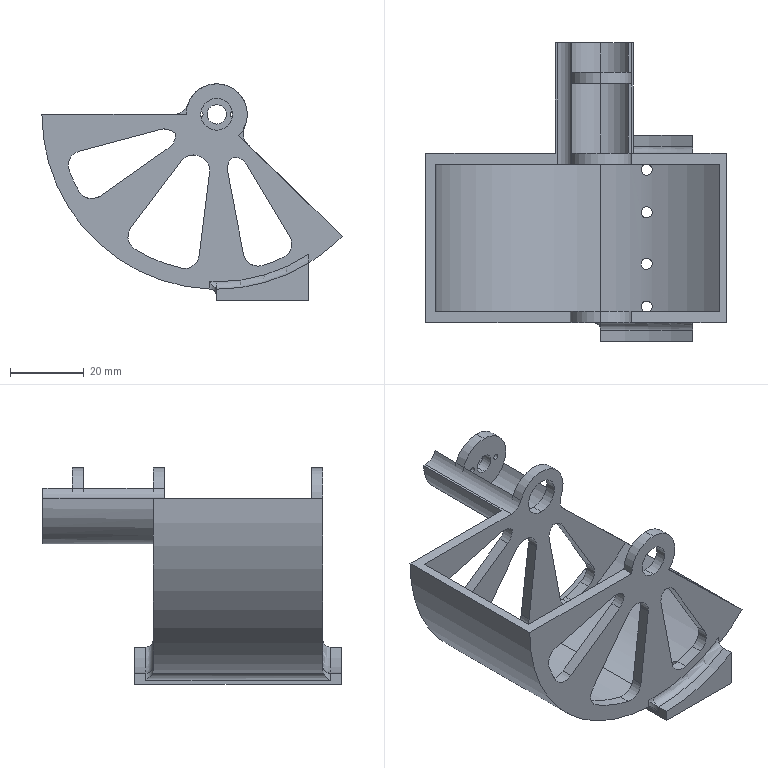Part | STEP file | Peel friction cover | 1 solid | 110 faces | box 81.568 x 81 x 58.817 mm | volume 32383 mm3 | cylinder 80 | plane 27 | torus 3 | commonest cylinder face diameters 8 x33 16.634 x9 3 x8 85.757 x6 1.6 x4 90 x4